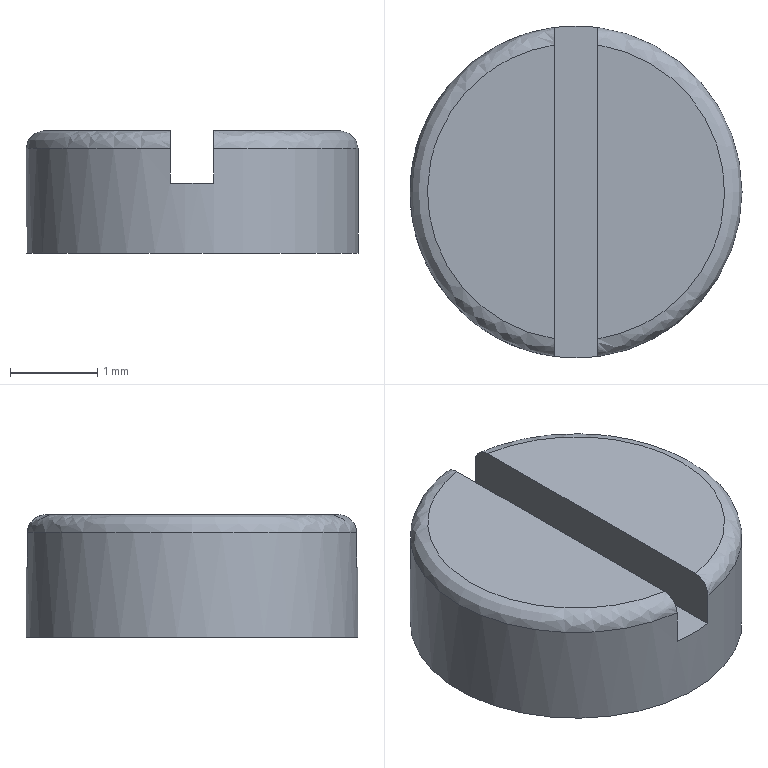Part | NX | 1 solid | 9 faces | box 3.8 x 3.8 x 1.4 mm | volume 14.641 mm3 | plane 6 | spline 2 | cylinder 1 | commonest cylinder face diameters 3.8 x1
STEP:
#1=CARTESIAN_POINT('',(1.9,0.,0.));
#2=VERTEX_POINT('',#1);
#3=CARTESIAN_POINT('',(0.,0.,0.));
#4=DIRECTION('',(0.,0.,1.));
#5=DIRECTION('',(1.,0.,0.));
#6=AXIS2_PLACEMENT_3D('',#3,#4,#5);
#7=CIRCLE('',#6,1.9);
#8=EDGE_CURVE('',#2,#2,#7,.T.);
#9=ORIENTED_EDGE('',*,*,#8,.T.);
#10=EDGE_LOOP('',(#9));
#11=FACE_BOUND('',#10,.T.);
#12=CARTESIAN_POINT('',(-0.25,1.883,1.2));
#13=VERTEX_POINT('',#12);
#14=CARTESIAN_POINT('',(-0.25,1.883,0.8));
#15=VERTEX_POINT('',#14);
#16=CARTESIAN_POINT('',(-0.25,1.883,1.4));
#17=DIRECTION('',(0.,0.,1.));
#18=VECTOR('',#17,1000.);
#19=LINE('',#16,#18);
#20=EDGE_CURVE('',#13,#15,#19,.F.);
#21=ORIENTED_EDGE('',*,*,#20,.T.);
#22=CARTESIAN_POINT('',(0.25,1.883,0.8));
#23=VERTEX_POINT('',#22);
#24=CARTESIAN_POINT('',(0.,0.,0.8));
#25=DIRECTION('',(0.,0.,1.));
#26=DIRECTION('',(1.,0.,0.));
#27=AXIS2_PLACEMENT_3D('',#24,#25,#26);
#28=CIRCLE('',#27,1.9);
#29=EDGE_CURVE('',#23,#15,#28,.T.);
#30=ORIENTED_EDGE('',*,*,#29,.F.);
#31=CARTESIAN_POINT('',(0.25,1.883,1.2));
#32=VERTEX_POINT('',#31);
#33=CARTESIAN_POINT('',(0.25,1.883,1.4));
#34=DIRECTION('',(0.,0.,-1.));
#35=VECTOR('',#34,1000.);
#36=LINE('',#33,#35);
#37=EDGE_CURVE('',#23,#32,#36,.F.);
#38=ORIENTED_EDGE('',*,*,#37,.T.);
#39=CARTESIAN_POINT('',(0.25,-1.883,1.2));
#40=VERTEX_POINT('',#39);
#41=CARTESIAN_POINT('',(0.,0.,1.2));
#42=DIRECTION('',(0.,0.,1.));
#43=DIRECTION('',(1.,0.,0.));
#44=AXIS2_PLACEMENT_3D('',#41,#42,#43);
#45=CIRCLE('',#44,1.9);
#46=EDGE_CURVE('',#32,#40,#45,.F.);
#47=ORIENTED_EDGE('',*,*,#46,.T.);
#48=CARTESIAN_POINT('',(0.25,-1.883,0.8));
#49=VERTEX_POINT('',#48);
#50=CARTESIAN_POINT('',(0.25,-1.883,1.4));
#51=DIRECTION('',(0.,0.,-1.));
#52=VECTOR('',#51,1000.);
#53=LINE('',#50,#52);
#54=EDGE_CURVE('',#40,#49,#53,.T.);
#55=ORIENTED_EDGE('',*,*,#54,.T.);
#56=CARTESIAN_POINT('',(-0.25,-1.883,0.8));
#57=VERTEX_POINT('',#56);
#58=CARTESIAN_POINT('',(0.,0.,0.8));
#59=DIRECTION('',(0.,0.,1.));
#60=DIRECTION('',(1.,0.,0.));
#61=AXIS2_PLACEMENT_3D('',#58,#59,#60);
#62=CIRCLE('',#61,1.9);
#63=EDGE_CURVE('',#57,#49,#62,.T.);
#64=ORIENTED_EDGE('',*,*,#63,.F.);
#65=CARTESIAN_POINT('',(-0.25,-1.883,1.2));
#66=VERTEX_POINT('',#65);
#67=CARTESIAN_POINT('',(-0.25,-1.883,1.4));
#68=DIRECTION('',(0.,0.,1.));
#69=VECTOR('',#68,1000.);
#70=LINE('',#67,#69);
#71=EDGE_CURVE('',#57,#66,#70,.T.);
#72=ORIENTED_EDGE('',*,*,#71,.T.);
#73=CARTESIAN_POINT('',(0.,0.,1.2));
#74=DIRECTION('',(0.,0.,1.));
#75=DIRECTION('',(1.,0.,0.));
#76=AXIS2_PLACEMENT_3D('',#73,#74,#75);
#77=CIRCLE('',#76,1.9);
#78=EDGE_CURVE('',#66,#13,#77,.F.);
#79=ORIENTED_EDGE('',*,*,#78,.T.);
#80=EDGE_LOOP('',(#21,#30,#38,#47,#55,#64,#72,#79));
#81=FACE_BOUND('',#80,.T.);
#82=CARTESIAN_POINT('',(0.,0.,0.));
#83=DIRECTION('',(0.,0.,1.));
#84=DIRECTION('',(1.,0.,0.));
#85=AXIS2_PLACEMENT_3D('',#82,#83,#84);
#86=CYLINDRICAL_SURFACE('',#85,1.9);
#87=ADVANCED_FACE('',(#11,#81),#86,.T.);
#88=ORIENTED_EDGE('',*,*,#8,.F.);
#89=EDGE_LOOP('',(#88));
#90=FACE_BOUND('',#89,.T.);
#91=CARTESIAN_POINT('',(0.,0.,0.));
#92=DIRECTION('',(0.,0.,-1.));
#93=DIRECTION('',(-1.,0.,0.));
#94=AXIS2_PLACEMENT_3D('',#91,#92,#93);
#95=PLANE('',#94);
#96=ADVANCED_FACE('',(#90),#95,.T.);
#97=CARTESIAN_POINT('',(-0.25,-1.682,1.4));
#98=VERTEX_POINT('',#97);
#99=CARTESIAN_POINT('',(-0.25,-1.883,1.2));
#100=CARTESIAN_POINT('',(-0.25,-1.883,1.306));
#101=CARTESIAN_POINT('',(-0.25,-1.788,1.4));
#102=CARTESIAN_POINT('',(-0.25,-1.682,1.4));
#103=B_SPLINE_CURVE_WITH_KNOTS('',3,(#99,#100,#101,#102),.UNSPECIFIED.,.F.,.F.,(4,4),(0.,0.000314),.UNSPECIFIED.);
#104=EDGE_CURVE('',#66,#98,#103,.T.);
#105=ORIENTED_EDGE('',*,*,#104,.T.);
#106=CARTESIAN_POINT('',(-0.25,1.682,1.4));
#107=VERTEX_POINT('',#106);
#108=CARTESIAN_POINT('',(-0.25,-1.682,1.4));
#109=CARTESIAN_POINT('',(-0.64,-1.623,1.4));
#110=CARTESIAN_POINT('',(-1.405,-1.207,1.4));
#111=CARTESIAN_POINT('',(-1.848,-0.00001373,1.4));
#112=CARTESIAN_POINT('',(-1.405,1.208,1.4));
#113=CARTESIAN_POINT('',(-0.6407,1.623,1.4));
#114=CARTESIAN_POINT('',(-0.25,1.682,1.4));
#115=B_SPLINE_CURVE_WITH_KNOTS('',3,(#108,#109,#110,#111,#112,#113,#114),.UNSPECIFIED.,.F.,.F.,(4,1,1,1,4),(0.,0.25,0.5,0.75,1.),.UNSPECIFIED.);
#116=EDGE_CURVE('',#98,#107,#115,.T.);
#117=ORIENTED_EDGE('',*,*,#116,.T.);
#118=CARTESIAN_POINT('',(-0.25,1.682,1.4));
#119=CARTESIAN_POINT('',(-0.25,1.788,1.4));
#120=CARTESIAN_POINT('',(-0.25,1.883,1.306));
#121=CARTESIAN_POINT('',(-0.25,1.883,1.2));
#122=B_SPLINE_CURVE_WITH_KNOTS('',3,(#118,#119,#120,#121),.UNSPECIFIED.,.F.,.F.,(4,4),(0.,0.000314),.UNSPECIFIED.);
#123=EDGE_CURVE('',#107,#13,#122,.T.);
#124=ORIENTED_EDGE('',*,*,#123,.T.);
#125=ORIENTED_EDGE('',*,*,#78,.F.);
#126=EDGE_LOOP('',(#105,#117,#124,#125));
#127=FACE_BOUND('',#126,.T.);
#128=CARTESIAN_POINT('',(-0.2174,-1.888,1.2));
#129=CARTESIAN_POINT('',(-3.269,-1.536,1.2));
#130=CARTESIAN_POINT('',(-3.269,1.536,1.2));
#131=CARTESIAN_POINT('',(-0.2174,1.888,1.2));
#132=CARTESIAN_POINT('',(-0.2174,-1.888,1.305));
#133=CARTESIAN_POINT('',(-3.269,-1.536,1.305));
#134=CARTESIAN_POINT('',(-3.269,1.536,1.305));
#135=CARTESIAN_POINT('',(-0.2174,1.888,1.305));
#136=CARTESIAN_POINT('',(-0.2065,-1.793,1.4));
#137=CARTESIAN_POINT('',(-3.105,-1.459,1.4));
#138=CARTESIAN_POINT('',(-3.105,1.459,1.4));
#139=CARTESIAN_POINT('',(-0.2065,1.793,1.4));
#140=CARTESIAN_POINT('',(-0.1946,-1.689,1.4));
#141=CARTESIAN_POINT('',(-2.925,-1.374,1.4));
#142=CARTESIAN_POINT('',(-2.925,1.374,1.4));
#143=CARTESIAN_POINT('',(-0.1946,1.689,1.4));
#144=(BOUNDED_SURFACE()B_SPLINE_SURFACE(3,3,((#128,#129,#130,#131),(#132,#133,#134,#135),(#136,#137,#138,#139),(#140,#141,#142,#143)),.SURF_OF_REVOLUTION.,.F.,.F.,.F.)B_SPLINE_SURFACE_WITH_KNOTS((4,4),(4,4),(0.,1.571),(0.,1.),.PIECEWISE_BEZIER_KNOTS.)GEOMETRIC_REPRESENTATION_ITEM()RATIONAL_B_SPLINE_SURFACE(((1.,0.4096,0.4096,1.),(1.,0.4096,0.4096,1.),(1.,0.4096,0.4096,1.),(1.,0.4096,0.4096,1.)))REPRESENTATION_ITEM('')SURFACE());
#145=ADVANCED_FACE('',(#127),#144,.T.);
#146=CARTESIAN_POINT('',(0.25,-1.682,1.4));
#147=VERTEX_POINT('',#146);
#148=CARTESIAN_POINT('',(0.25,-1.682,1.4));
#149=CARTESIAN_POINT('',(0.25,-1.788,1.4));
#150=CARTESIAN_POINT('',(0.25,-1.883,1.306));
#151=CARTESIAN_POINT('',(0.25,-1.883,1.2));
#152=B_SPLINE_CURVE_WITH_KNOTS('',3,(#148,#149,#150,#151),.UNSPECIFIED.,.F.,.F.,(4,4),(0.,0.000314),.UNSPECIFIED.);
#153=EDGE_CURVE('',#147,#40,#152,.T.);
#154=ORIENTED_EDGE('',*,*,#153,.T.);
#155=ORIENTED_EDGE('',*,*,#46,.F.);
#156=CARTESIAN_POINT('',(0.25,1.682,1.4));
#157=VERTEX_POINT('',#156);
#158=CARTESIAN_POINT('',(0.25,1.883,1.2));
#159=CARTESIAN_POINT('',(0.25,1.883,1.306));
#160=CARTESIAN_POINT('',(0.25,1.788,1.4));
#161=CARTESIAN_POINT('',(0.25,1.682,1.4));
#162=B_SPLINE_CURVE_WITH_KNOTS('',3,(#158,#159,#160,#161),.UNSPECIFIED.,.F.,.F.,(4,4),(0.,0.000314),.UNSPECIFIED.);
#163=EDGE_CURVE('',#32,#157,#162,.T.);
#164=ORIENTED_EDGE('',*,*,#163,.T.);
#165=CARTESIAN_POINT('',(0.25,1.682,1.4));
#166=CARTESIAN_POINT('',(0.64,1.623,1.4));
#167=CARTESIAN_POINT('',(1.405,1.207,1.4));
#168=CARTESIAN_POINT('',(1.848,0.00001373,1.4));
#169=CARTESIAN_POINT('',(1.405,-1.208,1.4));
#170=CARTESIAN_POINT('',(0.6407,-1.623,1.4));
#171=CARTESIAN_POINT('',(0.25,-1.682,1.4));
#172=B_SPLINE_CURVE_WITH_KNOTS('',3,(#165,#166,#167,#168,#169,#170,#171),.UNSPECIFIED.,.F.,.F.,(4,1,1,1,4),(0.,0.25,0.5,0.75,1.),.UNSPECIFIED.);
#173=EDGE_CURVE('',#157,#147,#172,.T.);
#174=ORIENTED_EDGE('',*,*,#173,.T.);
#175=EDGE_LOOP('',(#154,#155,#164,#174));
#176=FACE_BOUND('',#175,.T.);
#177=CARTESIAN_POINT('',(0.2174,1.888,1.2));
#178=CARTESIAN_POINT('',(3.269,1.536,1.2));
#179=CARTESIAN_POINT('',(3.269,-1.536,1.2));
#180=CARTESIAN_POINT('',(0.2174,-1.888,1.2));
#181=CARTESIAN_POINT('',(0.2174,1.888,1.305));
#182=CARTESIAN_POINT('',(3.269,1.536,1.305));
#183=CARTESIAN_POINT('',(3.269,-1.536,1.305));
#184=CARTESIAN_POINT('',(0.2174,-1.888,1.305));
#185=CARTESIAN_POINT('',(0.2065,1.793,1.4));
#186=CARTESIAN_POINT('',(3.105,1.459,1.4));
#187=CARTESIAN_POINT('',(3.105,-1.459,1.4));
#188=CARTESIAN_POINT('',(0.2065,-1.793,1.4));
#189=CARTESIAN_POINT('',(0.1946,1.689,1.4));
#190=CARTESIAN_POINT('',(2.925,1.374,1.4));
#191=CARTESIAN_POINT('',(2.925,-1.374,1.4));
#192=CARTESIAN_POINT('',(0.1946,-1.689,1.4));
#193=(BOUNDED_SURFACE()B_SPLINE_SURFACE(3,3,((#177,#178,#179,#180),(#181,#182,#183,#184),(#185,#186,#187,#188),(#189,#190,#191,#192)),.SURF_OF_REVOLUTION.,.F.,.F.,.F.)B_SPLINE_SURFACE_WITH_KNOTS((4,4),(4,4),(0.,1.571),(0.,1.),.PIECEWISE_BEZIER_KNOTS.)GEOMETRIC_REPRESENTATION_ITEM()RATIONAL_B_SPLINE_SURFACE(((1.,0.4096,0.4096,1.),(1.,0.4096,0.4096,1.),(1.,0.4096,0.4096,1.),(1.,0.4096,0.4096,1.)))REPRESENTATION_ITEM('')SURFACE());
#194=ADVANCED_FACE('',(#176),#193,.T.);
#195=ORIENTED_EDGE('',*,*,#116,.F.);
#196=CARTESIAN_POINT('',(-0.25,0.,1.4));
#197=DIRECTION('',(0.,1.,0.));
#198=VECTOR('',#197,1000.);
#199=LINE('',#196,#198);
#200=EDGE_CURVE('',#107,#98,#199,.F.);
#201=ORIENTED_EDGE('',*,*,#200,.F.);
#202=EDGE_LOOP('',(#195,#201));
#203=FACE_BOUND('',#202,.T.);
#204=CARTESIAN_POINT('',(0.,0.,1.4));
#205=DIRECTION('',(0.,0.,-1.));
#206=DIRECTION('',(-1.,0.,0.));
#207=AXIS2_PLACEMENT_3D('',#204,#205,#206);
#208=PLANE('',#207);
#209=ADVANCED_FACE('',(#203),#208,.F.);
#210=ORIENTED_EDGE('',*,*,#173,.F.);
#211=CARTESIAN_POINT('',(0.25,0.,1.4));
#212=DIRECTION('',(0.,1.,0.));
#213=VECTOR('',#212,1000.);
#214=LINE('',#211,#213);
#215=EDGE_CURVE('',#147,#157,#214,.T.);
#216=ORIENTED_EDGE('',*,*,#215,.F.);
#217=EDGE_LOOP('',(#210,#216));
#218=FACE_BOUND('',#217,.T.);
#219=CARTESIAN_POINT('',(0.,0.,1.4));
#220=DIRECTION('',(0.,0.,-1.));
#221=DIRECTION('',(-1.,0.,0.));
#222=AXIS2_PLACEMENT_3D('',#219,#220,#221);
#223=PLANE('',#222);
#224=ADVANCED_FACE('',(#218),#223,.F.);
#225=ORIENTED_EDGE('',*,*,#123,.F.);
#226=ORIENTED_EDGE('',*,*,#200,.T.);
#227=ORIENTED_EDGE('',*,*,#104,.F.);
#228=ORIENTED_EDGE('',*,*,#71,.F.);
#229=CARTESIAN_POINT('',(-0.25,3.,0.8));
#230=DIRECTION('',(0.,1.,0.));
#231=VECTOR('',#230,1000.);
#232=LINE('',#229,#231);
#233=EDGE_CURVE('',#15,#57,#232,.F.);
#234=ORIENTED_EDGE('',*,*,#233,.F.);
#235=ORIENTED_EDGE('',*,*,#20,.F.);
#236=EDGE_LOOP('',(#225,#226,#227,#228,#234,#235));
#237=FACE_BOUND('',#236,.T.);
#238=CARTESIAN_POINT('',(-0.25,3.,1.4));
#239=DIRECTION('',(-1.,0.,0.));
#240=DIRECTION('',(0.,0.,1.));
#241=AXIS2_PLACEMENT_3D('',#238,#239,#240);
#242=PLANE('',#241);
#243=ADVANCED_FACE('',(#237),#242,.F.);
#244=CARTESIAN_POINT('',(0.25,-3.,0.8));
#245=DIRECTION('',(0.,1.,0.));
#246=VECTOR('',#245,1000.);
#247=LINE('',#244,#246);
#248=EDGE_CURVE('',#49,#23,#247,.T.);
#249=ORIENTED_EDGE('',*,*,#248,.F.);
#250=ORIENTED_EDGE('',*,*,#54,.F.);
#251=ORIENTED_EDGE('',*,*,#153,.F.);
#252=ORIENTED_EDGE('',*,*,#215,.T.);
#253=ORIENTED_EDGE('',*,*,#163,.F.);
#254=ORIENTED_EDGE('',*,*,#37,.F.);
#255=EDGE_LOOP('',(#249,#250,#251,#252,#253,#254));
#256=FACE_BOUND('',#255,.T.);
#257=CARTESIAN_POINT('',(0.25,-3.,1.4));
#258=DIRECTION('',(1.,0.,0.));
#259=DIRECTION('',(0.,0.,-1.));
#260=AXIS2_PLACEMENT_3D('',#257,#258,#259);
#261=PLANE('',#260);
#262=ADVANCED_FACE('',(#256),#261,.F.);
#263=ORIENTED_EDGE('',*,*,#63,.T.);
#264=ORIENTED_EDGE('',*,*,#248,.T.);
#265=ORIENTED_EDGE('',*,*,#29,.T.);
#266=ORIENTED_EDGE('',*,*,#233,.T.);
#267=EDGE_LOOP('',(#263,#264,#265,#266));
#268=FACE_BOUND('',#267,.T.);
#269=CARTESIAN_POINT('',(0.,0.,0.8));
#270=DIRECTION('',(0.,0.,1.));
#271=DIRECTION('',(1.,0.,0.));
#272=AXIS2_PLACEMENT_3D('',#269,#270,#271);
#273=PLANE('',#272);
#274=ADVANCED_FACE('',(#268),#273,.T.);
#275=CLOSED_SHELL('',(#87,#96,#145,#194,#209,#224,#243,#262,#274));
#276=MANIFOLD_SOLID_BREP('',#275);
#277=(LENGTH_UNIT()NAMED_UNIT(*)SI_UNIT(.MILLI.,.METRE.));
#278=UNCERTAINTY_MEASURE_WITH_UNIT(LENGTH_MEASURE(0.0508),#277,'','');
#279=(NAMED_UNIT(*)PLANE_ANGLE_UNIT()SI_UNIT($,.RADIAN.));
#280=(NAMED_UNIT(*)SI_UNIT($,.STERADIAN.)SOLID_ANGLE_UNIT());
#281=(GEOMETRIC_REPRESENTATION_CONTEXT(3)GLOBAL_UNCERTAINTY_ASSIGNED_CONTEXT((#278))GLOBAL_UNIT_ASSIGNED_CONTEXT((#277,#279,#280))REPRESENTATION_CONTEXT('',''));
#282=ADVANCED_BREP_SHAPE_REPRESENTATION('',(#276),#281);